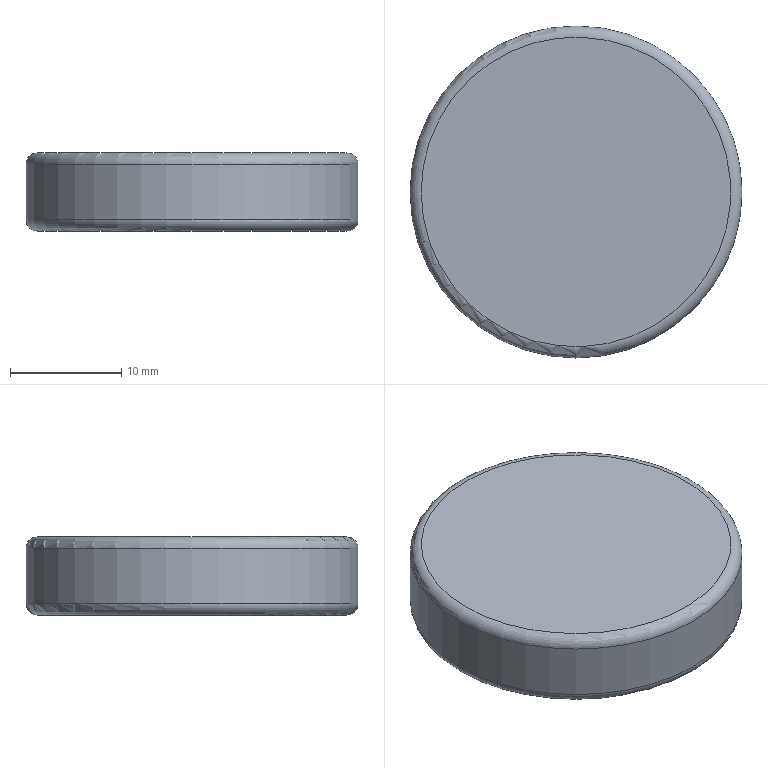Part | STEP file | CMT7E v7 | 1 solid | 5 faces | box 29.77 x 29.77 x 7 mm | volume 4833 mm3 | plane 2 | torus 2 | cylinder 1 | commonest cylinder face diameters 29.77 x1
STEP:
#1=CARTESIAN_POINT('',(0.,0.,0.));
#2=DIRECTION('',(0.,0.,1.));
#3=DIRECTION('',(1.,0.,0.));
#4=AXIS2_PLACEMENT_3D('',#1,#2,#3);
#5=CARTESIAN_POINT('',(-13.885,-39.,280.));
#6=VERTEX_POINT('',#5);
#7=CARTESIAN_POINT('',(0.,-39.,280.));
#8=DIRECTION('',(0.,0.,-1.));
#9=DIRECTION('',(-1.,0.,0.));
#10=AXIS2_PLACEMENT_3D('',#7,#8,#9);
#11=CIRCLE('',#10,13.885);
#12=CARTESIAN_POINT('',(0.,-39.,280.));
#13=DIRECTION('',(0.,0.,1.));
#14=DIRECTION('',(-1.,0.,0.));
#15=AXIS2_PLACEMENT_3D('',#12,#13,#14);
#16=PLANE('',#15);
#17=CARTESIAN_POINT('',(13.885,0.));
#18=CARTESIAN_POINT('',(13.885,-24.049));
#19=CARTESIAN_POINT('',(-6.942,-12.025));
#20=CARTESIAN_POINT('',(-27.77,0.));
#21=CARTESIAN_POINT('',(-6.942,12.025));
#22=CARTESIAN_POINT('',(13.885,24.049));
#23=CARTESIAN_POINT('',(13.885,0.));
#24=(BOUNDED_CURVE()B_SPLINE_CURVE(2,(#17,#18,#19,#20,#21,#22,#23),.UNSPECIFIED.,.T.,.F.)B_SPLINE_CURVE_WITH_KNOTS((1,2,2,2,2,1),(-2.094,0.,2.094,4.189,6.283,8.378),.UNSPECIFIED.)CURVE()GEOMETRIC_REPRESENTATION_ITEM()RATIONAL_B_SPLINE_CURVE((1.,0.5,1.,0.5,1.,0.5,1.))REPRESENTATION_ITEM(''));
#25=(GEOMETRIC_REPRESENTATION_CONTEXT(2)PARAMETRIC_REPRESENTATION_CONTEXT()REPRESENTATION_CONTEXT('',''));
#26=DEFINITIONAL_REPRESENTATION('',(#24),#25);
#27=PCURVE('',#16,#26);
#28=CARTESIAN_POINT('',(0.,-39.,279.));
#29=DIRECTION('',(0.,0.,1.));
#30=DIRECTION('',(1.,0.,0.));
#31=AXIS2_PLACEMENT_3D('',#28,#29,#30);
#32=TOROIDAL_SURFACE('',#31,13.885,1.);
#33=CARTESIAN_POINT('',(9.425,1.571));
#34=DIRECTION('',(-1.,0.));
#35=VECTOR('',#34,1.);
#36=LINE('',#33,#35);
#37=(GEOMETRIC_REPRESENTATION_CONTEXT(2)PARAMETRIC_REPRESENTATION_CONTEXT()REPRESENTATION_CONTEXT('',''));
#38=DEFINITIONAL_REPRESENTATION('',(#36),#37);
#39=PCURVE('',#32,#38);
#40=SURFACE_CURVE('',#11,(#27,#39),.PCURVE_S1.);
#41=EDGE_CURVE('',#6,#6,#40,.T.);
#42=ORIENTED_EDGE('',*,*,#41,.F.);
#43=EDGE_LOOP('',(#42));
#44=FACE_BOUND('',#43,.T.);
#45=ADVANCED_FACE('',(#44),#16,.T.);
#46=CARTESIAN_POINT('',(-14.885,-39.,279.));
#47=VERTEX_POINT('',#46);
#48=CARTESIAN_POINT('',(0.,-39.,279.));
#49=DIRECTION('',(0.,0.,1.));
#50=DIRECTION('',(-1.,0.,0.));
#51=AXIS2_PLACEMENT_3D('',#48,#49,#50);
#52=CIRCLE('',#51,14.885);
#53=CARTESIAN_POINT('',(3.142,0.));
#54=DIRECTION('',(1.,0.));
#55=VECTOR('',#54,1.);
#56=LINE('',#53,#55);
#57=(GEOMETRIC_REPRESENTATION_CONTEXT(2)PARAMETRIC_REPRESENTATION_CONTEXT()REPRESENTATION_CONTEXT('',''));
#58=DEFINITIONAL_REPRESENTATION('',(#56),#57);
#59=PCURVE('',#32,#58);
#60=CARTESIAN_POINT('',(0.,-39.,273.));
#61=DIRECTION('',(0.,0.,1.));
#62=DIRECTION('',(-1.,0.,0.));
#63=AXIS2_PLACEMENT_3D('',#60,#61,#62);
#64=CYLINDRICAL_SURFACE('',#63,14.885);
#65=CARTESIAN_POINT('',(0.,6.));
#66=DIRECTION('',(1.,0.));
#67=VECTOR('',#66,1.);
#68=LINE('',#65,#67);
#69=(GEOMETRIC_REPRESENTATION_CONTEXT(2)PARAMETRIC_REPRESENTATION_CONTEXT()REPRESENTATION_CONTEXT('',''));
#70=DEFINITIONAL_REPRESENTATION('',(#68),#69);
#71=PCURVE('',#64,#70);
#72=SURFACE_CURVE('',#52,(#59,#71),.PCURVE_S1.);
#73=EDGE_CURVE('',#47,#47,#72,.T.);
#74=ORIENTED_EDGE('',*,*,#73,.T.);
#75=CARTESIAN_POINT('',(-14.885,-39.,279.));
#76=CARTESIAN_POINT('',(-14.885,-39.,279.267));
#77=CARTESIAN_POINT('',(-14.8,-39.,279.528));
#78=CARTESIAN_POINT('',(-14.637,-39.,279.752));
#79=CARTESIAN_POINT('',(-14.413,-39.,279.915));
#80=CARTESIAN_POINT('',(-14.152,-39.,280.));
#81=CARTESIAN_POINT('',(-13.885,-39.,280.));
#82=(BOUNDED_CURVE()B_SPLINE_CURVE(6,(#75,#76,#77,#78,#79,#80,#81),.UNSPECIFIED.,.F.,.F.)B_SPLINE_CURVE_WITH_KNOTS((7,7),(0.,1.571),.PIECEWISE_BEZIER_KNOTS.)CURVE()GEOMETRIC_REPRESENTATION_ITEM()RATIONAL_B_SPLINE_CURVE((1.031,1.01,0.9979,0.994,0.9979,1.01,1.031))REPRESENTATION_ITEM(''));
#83=CARTESIAN_POINT('',(9.425,0.));
#84=DIRECTION('',(0.,1.));
#85=VECTOR('',#84,1.);
#86=LINE('',#83,#85);
#87=(GEOMETRIC_REPRESENTATION_CONTEXT(2)PARAMETRIC_REPRESENTATION_CONTEXT()REPRESENTATION_CONTEXT('',''));
#88=DEFINITIONAL_REPRESENTATION('',(#86),#87);
#89=PCURVE('',#32,#88);
#90=CARTESIAN_POINT('',(3.142,0.));
#91=DIRECTION('',(0.,1.));
#92=VECTOR('',#91,1.);
#93=LINE('',#90,#92);
#94=(GEOMETRIC_REPRESENTATION_CONTEXT(2)PARAMETRIC_REPRESENTATION_CONTEXT()REPRESENTATION_CONTEXT('',''));
#95=DEFINITIONAL_REPRESENTATION('',(#93),#94);
#96=PCURVE('',#32,#95);
#97=SEAM_CURVE('',#82,(#89,#96),.PCURVE_S1.);
#98=EDGE_CURVE('',#47,#6,#97,.T.);
#99=ORIENTED_EDGE('',*,*,#98,.T.);
#100=ORIENTED_EDGE('',*,*,#41,.T.);
#101=ORIENTED_EDGE('',*,*,#98,.F.);
#102=EDGE_LOOP('',(#74,#99,#100,#101));
#103=FACE_BOUND('',#102,.T.);
#104=ADVANCED_FACE('',(#103),#32,.T.);
#105=CARTESIAN_POINT('',(-13.885,-39.,273.));
#106=VERTEX_POINT('',#105);
#107=CARTESIAN_POINT('',(0.,-39.,273.));
#108=DIRECTION('',(0.,0.,1.));
#109=DIRECTION('',(-1.,0.,0.));
#110=AXIS2_PLACEMENT_3D('',#107,#108,#109);
#111=CIRCLE('',#110,13.885);
#112=CARTESIAN_POINT('',(0.,-39.,273.));
#113=DIRECTION('',(0.,0.,1.));
#114=DIRECTION('',(-1.,0.,0.));
#115=AXIS2_PLACEMENT_3D('',#112,#113,#114);
#116=PLANE('',#115);
#117=CARTESIAN_POINT('',(0.,0.));
#118=DIRECTION('',(1.,0.));
#119=AXIS2_PLACEMENT_2D('',#117,#118);
#120=CIRCLE('',#119,13.885);
#121=(GEOMETRIC_REPRESENTATION_CONTEXT(2)PARAMETRIC_REPRESENTATION_CONTEXT()REPRESENTATION_CONTEXT('',''));
#122=DEFINITIONAL_REPRESENTATION('',(#120),#121);
#123=PCURVE('',#116,#122);
#124=CARTESIAN_POINT('',(0.,-39.,274.));
#125=DIRECTION('',(0.,0.,1.));
#126=DIRECTION('',(1.,0.,0.));
#127=AXIS2_PLACEMENT_3D('',#124,#125,#126);
#128=TOROIDAL_SURFACE('',#127,13.885,1.);
#129=CARTESIAN_POINT('',(3.142,4.712));
#130=DIRECTION('',(1.,0.));
#131=VECTOR('',#130,1.);
#132=LINE('',#129,#131);
#133=(GEOMETRIC_REPRESENTATION_CONTEXT(2)PARAMETRIC_REPRESENTATION_CONTEXT()REPRESENTATION_CONTEXT('',''));
#134=DEFINITIONAL_REPRESENTATION('',(#132),#133);
#135=PCURVE('',#128,#134);
#136=SURFACE_CURVE('',#111,(#123,#135),.PCURVE_S1.);
#137=EDGE_CURVE('',#106,#106,#136,.T.);
#138=ORIENTED_EDGE('',*,*,#137,.F.);
#139=EDGE_LOOP('',(#138));
#140=FACE_BOUND('',#139,.T.);
#141=ADVANCED_FACE('',(#140),#116,.F.);
#142=CARTESIAN_POINT('',(-14.885,-39.,274.));
#143=VERTEX_POINT('',#142);
#144=CARTESIAN_POINT('',(0.,-39.,274.));
#145=DIRECTION('',(0.,0.,-1.));
#146=DIRECTION('',(-1.,0.,0.));
#147=AXIS2_PLACEMENT_3D('',#144,#145,#146);
#148=CIRCLE('',#147,14.885);
#149=CARTESIAN_POINT('',(6.283,1.));
#150=DIRECTION('',(-1.,0.));
#151=VECTOR('',#150,1.);
#152=LINE('',#149,#151);
#153=(GEOMETRIC_REPRESENTATION_CONTEXT(2)PARAMETRIC_REPRESENTATION_CONTEXT()REPRESENTATION_CONTEXT('',''));
#154=DEFINITIONAL_REPRESENTATION('',(#152),#153);
#155=PCURVE('',#64,#154);
#156=CARTESIAN_POINT('',(9.425,6.283));
#157=DIRECTION('',(-1.,0.));
#158=VECTOR('',#157,1.);
#159=LINE('',#156,#158);
#160=(GEOMETRIC_REPRESENTATION_CONTEXT(2)PARAMETRIC_REPRESENTATION_CONTEXT()REPRESENTATION_CONTEXT('',''));
#161=DEFINITIONAL_REPRESENTATION('',(#159),#160);
#162=PCURVE('',#128,#161);
#163=SURFACE_CURVE('',#148,(#155,#162),.PCURVE_S1.);
#164=EDGE_CURVE('',#143,#143,#163,.T.);
#165=ORIENTED_EDGE('',*,*,#164,.F.);
#166=CARTESIAN_POINT('',(-14.885,-39.,274.));
#167=CARTESIAN_POINT('',(-14.885,-39.,279.));
#168=B_SPLINE_CURVE_WITH_KNOTS('',1,(#166,#167),.UNSPECIFIED.,.F.,.F.,(2,2),(1.,6.),.PIECEWISE_BEZIER_KNOTS.);
#169=CARTESIAN_POINT('',(6.283,0.));
#170=DIRECTION('',(0.,1.));
#171=VECTOR('',#170,1.);
#172=LINE('',#169,#171);
#173=(GEOMETRIC_REPRESENTATION_CONTEXT(2)PARAMETRIC_REPRESENTATION_CONTEXT()REPRESENTATION_CONTEXT('',''));
#174=DEFINITIONAL_REPRESENTATION('',(#172),#173);
#175=PCURVE('',#64,#174);
#176=CARTESIAN_POINT('',(0.,0.));
#177=DIRECTION('',(0.,1.));
#178=VECTOR('',#177,1.);
#179=LINE('',#176,#178);
#180=(GEOMETRIC_REPRESENTATION_CONTEXT(2)PARAMETRIC_REPRESENTATION_CONTEXT()REPRESENTATION_CONTEXT('',''));
#181=DEFINITIONAL_REPRESENTATION('',(#179),#180);
#182=PCURVE('',#64,#181);
#183=SEAM_CURVE('',#168,(#175,#182),.PCURVE_S1.);
#184=EDGE_CURVE('',#143,#47,#183,.T.);
#185=ORIENTED_EDGE('',*,*,#184,.T.);
#186=ORIENTED_EDGE('',*,*,#73,.F.);
#187=ORIENTED_EDGE('',*,*,#184,.F.);
#188=EDGE_LOOP('',(#165,#185,#186,#187));
#189=FACE_BOUND('',#188,.T.);
#190=ADVANCED_FACE('',(#189),#64,.T.);
#191=ORIENTED_EDGE('',*,*,#137,.T.);
#192=CARTESIAN_POINT('',(-13.885,-39.,273.));
#193=CARTESIAN_POINT('',(-14.152,-39.,273.));
#194=CARTESIAN_POINT('',(-14.413,-39.,273.085));
#195=CARTESIAN_POINT('',(-14.637,-39.,273.248));
#196=CARTESIAN_POINT('',(-14.8,-39.,273.472));
#197=CARTESIAN_POINT('',(-14.885,-39.,273.733));
#198=CARTESIAN_POINT('',(-14.885,-39.,274.));
#199=(BOUNDED_CURVE()B_SPLINE_CURVE(6,(#192,#193,#194,#195,#196,#197,#198),.UNSPECIFIED.,.F.,.F.)B_SPLINE_CURVE_WITH_KNOTS((7,7),(4.712,6.283),.PIECEWISE_BEZIER_KNOTS.)CURVE()GEOMETRIC_REPRESENTATION_ITEM()RATIONAL_B_SPLINE_CURVE((1.031,1.01,0.9979,0.994,0.9979,1.01,1.031))REPRESENTATION_ITEM(''));
#200=CARTESIAN_POINT('',(9.425,0.));
#201=DIRECTION('',(0.,1.));
#202=VECTOR('',#201,1.);
#203=LINE('',#200,#202);
#204=(GEOMETRIC_REPRESENTATION_CONTEXT(2)PARAMETRIC_REPRESENTATION_CONTEXT()REPRESENTATION_CONTEXT('',''));
#205=DEFINITIONAL_REPRESENTATION('',(#203),#204);
#206=PCURVE('',#128,#205);
#207=CARTESIAN_POINT('',(3.142,0.));
#208=DIRECTION('',(0.,1.));
#209=VECTOR('',#208,1.);
#210=LINE('',#207,#209);
#211=(GEOMETRIC_REPRESENTATION_CONTEXT(2)PARAMETRIC_REPRESENTATION_CONTEXT()REPRESENTATION_CONTEXT('',''));
#212=DEFINITIONAL_REPRESENTATION('',(#210),#211);
#213=PCURVE('',#128,#212);
#214=SEAM_CURVE('',#199,(#206,#213),.PCURVE_S1.);
#215=EDGE_CURVE('',#106,#143,#214,.T.);
#216=ORIENTED_EDGE('',*,*,#215,.T.);
#217=ORIENTED_EDGE('',*,*,#164,.T.);
#218=ORIENTED_EDGE('',*,*,#215,.F.);
#219=EDGE_LOOP('',(#191,#216,#217,#218));
#220=FACE_BOUND('',#219,.T.);
#221=ADVANCED_FACE('',(#220),#128,.T.);
#222=CLOSED_SHELL('',(#45,#104,#141,#190,#221));
#223=MANIFOLD_SOLID_BREP('',#222);
#224=(LENGTH_UNIT()NAMED_UNIT(*)SI_UNIT(.MILLI.,.METRE.));
#225=UNCERTAINTY_MEASURE_WITH_UNIT(LENGTH_MEASURE(0.0000002),#224,'','');
#226=(NAMED_UNIT(*)PLANE_ANGLE_UNIT()SI_UNIT($,.RADIAN.));
#227=(NAMED_UNIT(*)SI_UNIT($,.STERADIAN.)SOLID_ANGLE_UNIT());
#228=(GEOMETRIC_REPRESENTATION_CONTEXT(3)GLOBAL_UNCERTAINTY_ASSIGNED_CONTEXT((#225))GLOBAL_UNIT_ASSIGNED_CONTEXT((#224,#226,#227))REPRESENTATION_CONTEXT('',''));
#229=ADVANCED_BREP_SHAPE_REPRESENTATION('',(#4,#223),#228);